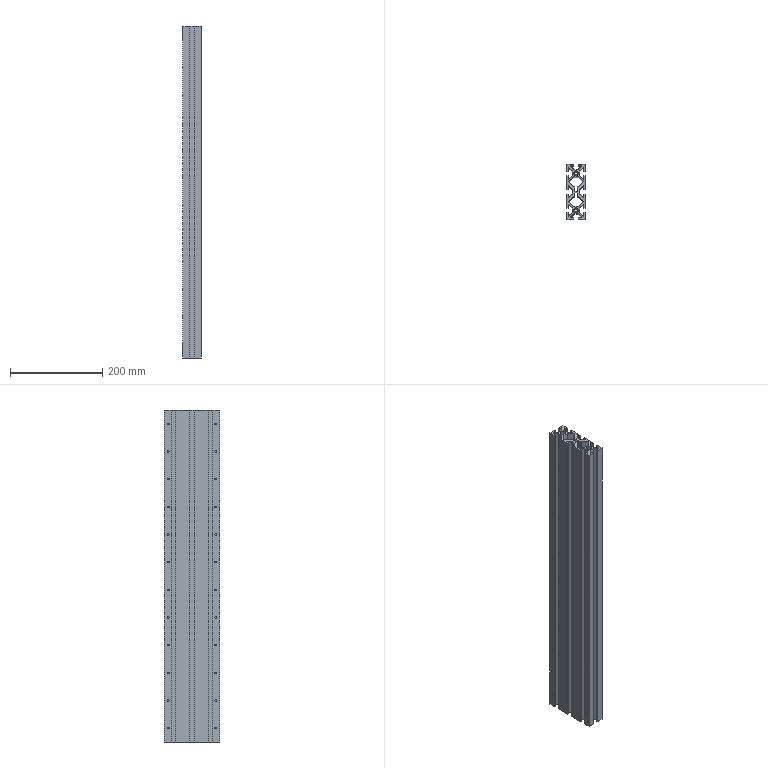Part | 1 solid | 210 faces | box 40 x 120 x 720 mm | volume 1551949 mm3 | cylinder 112 | plane 90 | cone 8 | commonest cylinder face diameters 3.3 x96 10.2 x8 3 x4 6.8 x4